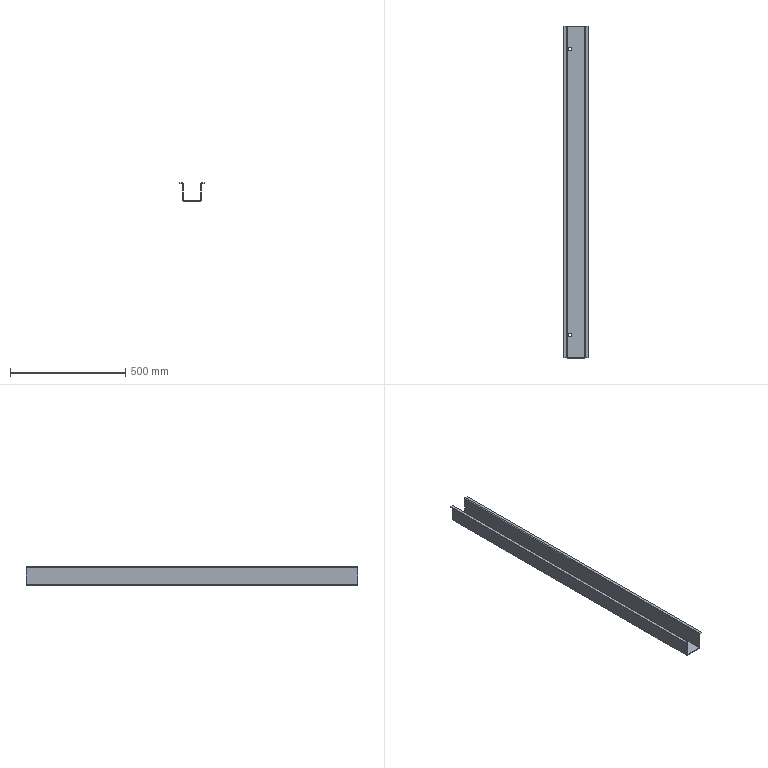Part | STEP file | 1 solid | 42 faces | box 104 x 1437 x 78 mm | volume 1081502 mm3 | plane 30 | cylinder 12 | commonest cylinder face diameters 0.4 x4 6.4 x4 15 x4